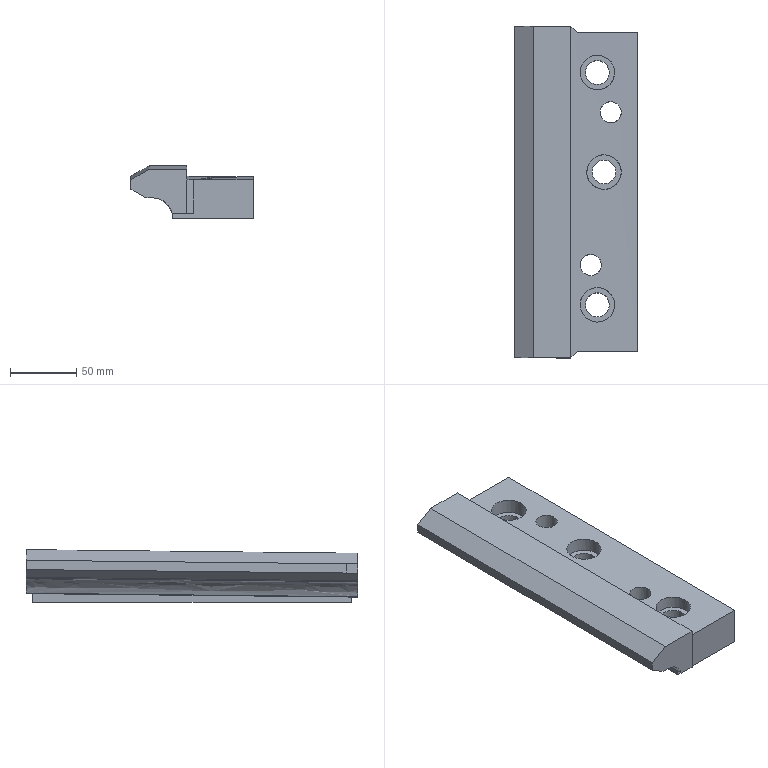Part | NX | features solid 2 | 1 solid | 33 faces | box 92.195 x 250 x 39.654 mm | volume 579481 mm3 | plane 14 | spline 11 | cylinder 8 | commonest cylinder face diameters 18 x3 26 x3 16 x2
STEP:
#1=CARTESIAN_POINT('',(719.105,10.,-45.));
#2=VERTEX_POINT('',#1);
#3=CARTESIAN_POINT('',(719.105,10.,-38.475));
#4=VERTEX_POINT('',#3);
#5=CARTESIAN_POINT('',(719.105,10.,-49.344));
#6=DIRECTION('',(0.,0.,-1.));
#7=VECTOR('',#6,1000.);
#8=LINE('',#5,#7);
#9=EDGE_CURVE('',#2,#4,#8,.F.);
#10=ORIENTED_EDGE('',*,*,#9,.F.);
#11=CARTESIAN_POINT('',(719.103,-230.,-45.));
#12=VERTEX_POINT('',#11);
#13=CARTESIAN_POINT('',(719.105,10.,-45.));
#14=CARTESIAN_POINT('',(719.108,-70.,-45.));
#15=CARTESIAN_POINT('',(719.097,-150.,-45.));
#16=CARTESIAN_POINT('',(719.103,-230.,-45.));
#17=B_SPLINE_CURVE_WITH_KNOTS('',3,(#13,#14,#15,#16),.UNSPECIFIED.,.F.,.F.,(4,4),(0.,0.24),.UNSPECIFIED.);
#18=EDGE_CURVE('',#2,#12,#17,.T.);
#19=ORIENTED_EDGE('',*,*,#18,.T.);
#20=CARTESIAN_POINT('',(719.103,-230.,-41.019));
#21=VERTEX_POINT('',#20);
#22=CARTESIAN_POINT('',(719.103,-230.,-50.615));
#23=DIRECTION('',(0.,0.,-1.));
#24=VECTOR('',#23,1000.);
#25=LINE('',#22,#24);
#26=EDGE_CURVE('',#21,#12,#25,.T.);
#27=ORIENTED_EDGE('',*,*,#26,.F.);
#28=CARTESIAN_POINT('',(719.103,-230.,-41.019));
#29=CARTESIAN_POINT('',(719.097,-149.999,-40.247));
#30=CARTESIAN_POINT('',(719.108,-69.999,-39.4));
#31=CARTESIAN_POINT('',(719.105,10.,-38.475));
#32=B_SPLINE_CURVE_WITH_KNOTS('',3,(#28,#29,#30,#31),.UNSPECIFIED.,.F.,.F.,(4,4),(0.006561,0.2466),.UNSPECIFIED.);
#33=EDGE_CURVE('',#21,#4,#32,.T.);
#34=ORIENTED_EDGE('',*,*,#33,.T.);
#35=EDGE_LOOP('',(#10,#19,#27,#34));
#36=FACE_BOUND('',#35,.T.);
#37=CARTESIAN_POINT('',(719.105,10.,-38.434));
#38=CARTESIAN_POINT('',(719.105,10.,-45.039));
#39=CARTESIAN_POINT('',(719.108,-70.005,-39.358));
#40=CARTESIAN_POINT('',(719.108,-70.005,-45.963));
#41=CARTESIAN_POINT('',(719.097,-149.999,-40.21));
#42=CARTESIAN_POINT('',(719.097,-149.999,-46.815));
#43=CARTESIAN_POINT('',(719.103,-230.,-40.978));
#44=CARTESIAN_POINT('',(719.103,-230.,-47.583));
#45=B_SPLINE_SURFACE_WITH_KNOTS('',3,1,((#37,#38),(#39,#40),(#41,#42),(#43,#44)),.SURF_OF_LINEAR_EXTRUSION.,.F.,.F.,.F.,(4,4),(2,2),(0.3477,0.6676),(0.,1.),.PIECEWISE_BEZIER_KNOTS.);
#46=ADVANCED_FACE('',(#36),#45,.F.);
#47=CARTESIAN_POINT('',(780.,10.,-45.));
#48=VERTEX_POINT('',#47);
#49=CARTESIAN_POINT('',(730.,10.,-45.));
#50=DIRECTION('',(1.,0.,0.));
#51=VECTOR('',#50,1000.);
#52=LINE('',#49,#51);
#53=EDGE_CURVE('',#2,#48,#52,.T.);
#54=ORIENTED_EDGE('',*,*,#53,.F.);
#55=ORIENTED_EDGE('',*,*,#9,.T.);
#56=CARTESIAN_POINT('',(718.904,10.,-38.359));
#57=VERTEX_POINT('',#56);
#58=CARTESIAN_POINT('',(719.105,10.,-38.475));
#59=CARTESIAN_POINT('',(719.038,10.,-38.437));
#60=CARTESIAN_POINT('',(718.971,10.,-38.398));
#61=CARTESIAN_POINT('',(718.904,10.,-38.359));
#62=B_SPLINE_CURVE_WITH_KNOTS('',3,(#58,#59,#60,#61),.UNSPECIFIED.,.F.,.F.,(4,4),(0.01267,0.0129),.UNSPECIFIED.);
#63=EDGE_CURVE('',#4,#57,#62,.T.);
#64=ORIENTED_EDGE('',*,*,#63,.T.);
#65=CARTESIAN_POINT('',(735.,10.,-38.359));
#66=VERTEX_POINT('',#65);
#67=CARTESIAN_POINT('',(669.104,10.,-38.359));
#68=DIRECTION('',(1.,0.,0.));
#69=VECTOR('',#68,1000.);
#70=LINE('',#67,#69);
#71=EDGE_CURVE('',#57,#66,#70,.T.);
#72=ORIENTED_EDGE('',*,*,#71,.T.);
#73=CARTESIAN_POINT('',(735.,10.,-13.527));
#74=VERTEX_POINT('',#73);
#75=CARTESIAN_POINT('',(735.,10.,-43.689));
#76=DIRECTION('',(0.,0.,-1.));
#77=VECTOR('',#76,1000.);
#78=LINE('',#75,#77);
#79=EDGE_CURVE('',#74,#66,#78,.T.);
#80=ORIENTED_EDGE('',*,*,#79,.F.);
#81=CARTESIAN_POINT('',(780.,10.,-13.527));
#82=VERTEX_POINT('',#81);
#83=CARTESIAN_POINT('',(754.976,10.,-13.527));
#84=DIRECTION('',(1.,0.,0.));
#85=VECTOR('',#84,1000.);
#86=LINE('',#83,#85);
#87=EDGE_CURVE('',#74,#82,#86,.T.);
#88=ORIENTED_EDGE('',*,*,#87,.T.);
#89=CARTESIAN_POINT('',(780.,10.,-5.));
#90=DIRECTION('',(0.,0.,1.));
#91=VECTOR('',#90,1000.);
#92=LINE('',#89,#91);
#93=EDGE_CURVE('',#48,#82,#92,.T.);
#94=ORIENTED_EDGE('',*,*,#93,.F.);
#95=EDGE_LOOP('',(#54,#55,#64,#72,#80,#88,#94));
#96=FACE_BOUND('',#95,.T.);
#97=CARTESIAN_POINT('',(730.,10.,-149.315));
#98=DIRECTION('',(0.,-1.,0.));
#99=DIRECTION('',(0.,0.,-1.));
#100=AXIS2_PLACEMENT_3D('',#97,#98,#99);
#101=PLANE('',#100);
#102=ADVANCED_FACE('',(#96),#101,.F.);
#103=CARTESIAN_POINT('',(780.,-230.,-45.));
#104=VERTEX_POINT('',#103);
#105=CARTESIAN_POINT('',(730.,-230.,-45.));
#106=DIRECTION('',(-1.,0.,0.));
#107=VECTOR('',#106,1000.);
#108=LINE('',#105,#107);
#109=EDGE_CURVE('',#104,#12,#108,.T.);
#110=ORIENTED_EDGE('',*,*,#109,.F.);
#111=CARTESIAN_POINT('',(780.,-230.,-16.093));
#112=VERTEX_POINT('',#111);
#113=CARTESIAN_POINT('',(780.,-230.,-5.));
#114=DIRECTION('',(0.,0.,-1.));
#115=VECTOR('',#114,1000.);
#116=LINE('',#113,#115);
#117=EDGE_CURVE('',#112,#104,#116,.T.);
#118=ORIENTED_EDGE('',*,*,#117,.F.);
#119=CARTESIAN_POINT('',(735.,-230.,-16.093));
#120=VERTEX_POINT('',#119);
#121=CARTESIAN_POINT('',(755.021,-230.,-16.093));
#122=DIRECTION('',(1.,0.,0.));
#123=VECTOR('',#122,1000.);
#124=LINE('',#121,#123);
#125=EDGE_CURVE('',#112,#120,#124,.F.);
#126=ORIENTED_EDGE('',*,*,#125,.T.);
#127=CARTESIAN_POINT('',(735.,-230.,-41.019));
#128=VERTEX_POINT('',#127);
#129=CARTESIAN_POINT('',(735.,-230.,-16.093));
#130=DIRECTION('',(0.,0.,1.));
#131=VECTOR('',#130,1000.);
#132=LINE('',#129,#131);
#133=EDGE_CURVE('',#128,#120,#132,.T.);
#134=ORIENTED_EDGE('',*,*,#133,.F.);
#135=CARTESIAN_POINT('',(669.103,-230.,-41.019));
#136=DIRECTION('',(1.,0.,0.));
#137=VECTOR('',#136,1000.);
#138=LINE('',#135,#137);
#139=EDGE_CURVE('',#21,#128,#138,.T.);
#140=ORIENTED_EDGE('',*,*,#139,.F.);
#141=ORIENTED_EDGE('',*,*,#26,.T.);
#142=EDGE_LOOP('',(#110,#118,#126,#134,#140,#141));
#143=FACE_BOUND('',#142,.T.);
#144=CARTESIAN_POINT('',(730.,-230.,49.361));
#145=DIRECTION('',(0.,1.,0.));
#146=DIRECTION('',(0.,0.,1.));
#147=AXIS2_PLACEMENT_3D('',#144,#145,#146);
#148=PLANE('',#147);
#149=ADVANCED_FACE('',(#143),#148,.F.);
#150=ORIENTED_EDGE('',*,*,#117,.T.);
#151=CARTESIAN_POINT('',(780.,-135.,-45.));
#152=DIRECTION('',(0.,1.,0.));
#153=VECTOR('',#152,1000.);
#154=LINE('',#151,#153);
#155=EDGE_CURVE('',#104,#48,#154,.T.);
#156=ORIENTED_EDGE('',*,*,#155,.T.);
#157=ORIENTED_EDGE('',*,*,#93,.T.);
#158=CARTESIAN_POINT('',(780.,10.,-13.527));
#159=CARTESIAN_POINT('',(780.,-69.999,-14.462));
#160=CARTESIAN_POINT('',(780.,-149.999,-15.327));
#161=CARTESIAN_POINT('',(780.,-230.,-16.093));
#162=B_SPLINE_CURVE_WITH_KNOTS('',3,(#158,#159,#160,#161),.UNSPECIFIED.,.F.,.F.,(4,4),(0.8306,1.071),.UNSPECIFIED.);
#163=EDGE_CURVE('',#82,#112,#162,.T.);
#164=ORIENTED_EDGE('',*,*,#163,.T.);
#165=EDGE_LOOP('',(#150,#156,#157,#164));
#166=FACE_BOUND('',#165,.T.);
#167=CARTESIAN_POINT('',(780.,-135.,-5.));
#168=DIRECTION('',(1.,0.,0.));
#169=DIRECTION('',(0.,1.,0.));
#170=AXIS2_PLACEMENT_3D('',#167,#168,#169);
#171=PLANE('',#170);
#172=ADVANCED_FACE('',(#166),#171,.T.);
#173=CARTESIAN_POINT('',(741.,-20.,-25.));
#174=VERTEX_POINT('',#173);
#175=CARTESIAN_POINT('',(750.,-20.,-25.));
#176=DIRECTION('',(0.,0.,-1.));
#177=DIRECTION('',(-1.,0.,0.));
#178=AXIS2_PLACEMENT_3D('',#175,#176,#177);
#179=CIRCLE('',#178,9.);
#180=EDGE_CURVE('',#174,#174,#179,.T.);
#181=ORIENTED_EDGE('',*,*,#180,.F.);
#182=EDGE_LOOP('',(#181));
#183=FACE_BOUND('',#182,.T.);
#184=CARTESIAN_POINT('',(741.,-20.,-45.));
#185=VERTEX_POINT('',#184);
#186=CARTESIAN_POINT('',(750.,-20.,-45.));
#187=DIRECTION('',(0.,0.,-1.));
#188=DIRECTION('',(-1.,0.,0.));
#189=AXIS2_PLACEMENT_3D('',#186,#187,#188);
#190=CIRCLE('',#189,9.);
#191=EDGE_CURVE('',#185,#185,#190,.F.);
#192=ORIENTED_EDGE('',*,*,#191,.F.);
#193=EDGE_LOOP('',(#192));
#194=FACE_BOUND('',#193,.T.);
#195=CARTESIAN_POINT('',(750.,-20.,-40.));
#196=DIRECTION('',(0.,0.,-1.));
#197=DIRECTION('',(-1.,0.,0.));
#198=AXIS2_PLACEMENT_3D('',#195,#196,#197);
#199=CYLINDRICAL_SURFACE('',#198,9.);
#200=ADVANCED_FACE('',(#183,#194),#199,.F.);
#201=CARTESIAN_POINT('',(752.044,-50.84,-14.225));
#202=VERTEX_POINT('',#201);
#203=CARTESIAN_POINT('',(754.43,-56.899,-14.293));
#204=CARTESIAN_POINT('',(751.181,-50.93,-14.226));
#205=CARTESIAN_POINT('',(753.11,-44.423,-14.153));
#206=CARTESIAN_POINT('',(759.063,-41.185,-14.116));
#207=CARTESIAN_POINT('',(765.573,-43.103,-14.138));
#208=CARTESIAN_POINT('',(768.815,-49.068,-14.205));
#209=CARTESIAN_POINT('',(766.898,-55.567,-14.278));
#210=CARTESIAN_POINT('',(760.941,-58.816,-14.314));
#211=CARTESIAN_POINT('',(754.43,-56.899,-14.293));
#212=CARTESIAN_POINT('',(751.181,-50.93,-14.226));
#213=CARTESIAN_POINT('',(753.11,-44.423,-14.153));
#214=B_SPLINE_CURVE_WITH_KNOTS('',3,(#203,#204,#205,#206,#207,#208,#209,#210,#211,#212,#213),.UNSPECIFIED.,.T.,.F.,(1,1,1,1,1,1,1,1,1,1,1,1,1,1,1),(-0.01876,-0.0125,-0.006252,0.,0.006252,0.0125,0.01876,0.02501,0.03126,0.03751,0.04377,0.05002,0.05627,0.06252,0.06878),.UNSPECIFIED.);
#215=EDGE_CURVE('',#202,#202,#214,.T.);
#216=ORIENTED_EDGE('',*,*,#215,.F.);
#217=EDGE_LOOP('',(#216));
#218=FACE_BOUND('',#217,.T.);
#219=CARTESIAN_POINT('',(752.,-50.,-45.));
#220=VERTEX_POINT('',#219);
#221=CARTESIAN_POINT('',(760.,-50.,-45.));
#222=DIRECTION('',(0.,0.,-1.));
#223=DIRECTION('',(-1.,0.,0.));
#224=AXIS2_PLACEMENT_3D('',#221,#222,#223);
#225=CIRCLE('',#224,8.);
#226=EDGE_CURVE('',#220,#220,#225,.F.);
#227=ORIENTED_EDGE('',*,*,#226,.F.);
#228=EDGE_LOOP('',(#227));
#229=FACE_BOUND('',#228,.T.);
#230=CARTESIAN_POINT('',(760.,-50.,-95.));
#231=DIRECTION('',(0.,0.,1.));
#232=DIRECTION('',(1.,0.,0.));
#233=AXIS2_PLACEMENT_3D('',#230,#231,#232);
#234=CYLINDRICAL_SURFACE('',#233,8.);
#235=ADVANCED_FACE('',(#218,#229),#234,.F.);
#236=CARTESIAN_POINT('',(746.,-95.,-25.));
#237=VERTEX_POINT('',#236);
#238=CARTESIAN_POINT('',(755.,-95.,-25.));
#239=DIRECTION('',(0.,0.,-1.));
#240=DIRECTION('',(-1.,0.,0.));
#241=AXIS2_PLACEMENT_3D('',#238,#239,#240);
#242=CIRCLE('',#241,9.);
#243=EDGE_CURVE('',#237,#237,#242,.T.);
#244=ORIENTED_EDGE('',*,*,#243,.F.);
#245=EDGE_LOOP('',(#244));
#246=FACE_BOUND('',#245,.T.);
#247=CARTESIAN_POINT('',(746.,-95.,-45.));
#248=VERTEX_POINT('',#247);
#249=CARTESIAN_POINT('',(755.,-95.,-45.));
#250=DIRECTION('',(0.,0.,-1.));
#251=DIRECTION('',(-1.,0.,0.));
#252=AXIS2_PLACEMENT_3D('',#249,#250,#251);
#253=CIRCLE('',#252,9.);
#254=EDGE_CURVE('',#248,#248,#253,.F.);
#255=ORIENTED_EDGE('',*,*,#254,.F.);
#256=EDGE_LOOP('',(#255));
#257=FACE_BOUND('',#256,.T.);
#258=CARTESIAN_POINT('',(755.,-95.,-40.));
#259=DIRECTION('',(0.,0.,-1.));
#260=DIRECTION('',(-1.,0.,0.));
#261=AXIS2_PLACEMENT_3D('',#258,#259,#260);
#262=CYLINDRICAL_SURFACE('',#261,9.);
#263=ADVANCED_FACE('',(#246,#257),#262,.F.);
#264=CARTESIAN_POINT('',(741.,-195.,-25.));
#265=VERTEX_POINT('',#264);
#266=CARTESIAN_POINT('',(750.,-195.,-25.));
#267=DIRECTION('',(0.,0.,-1.));
#268=DIRECTION('',(-1.,0.,0.));
#269=AXIS2_PLACEMENT_3D('',#266,#267,#268);
#270=CIRCLE('',#269,9.);
#271=EDGE_CURVE('',#265,#265,#270,.T.);
#272=ORIENTED_EDGE('',*,*,#271,.F.);
#273=EDGE_LOOP('',(#272));
#274=FACE_BOUND('',#273,.T.);
#275=CARTESIAN_POINT('',(741.,-195.,-45.));
#276=VERTEX_POINT('',#275);
#277=CARTESIAN_POINT('',(750.,-195.,-45.));
#278=DIRECTION('',(0.,0.,-1.));
#279=DIRECTION('',(-1.,0.,0.));
#280=AXIS2_PLACEMENT_3D('',#277,#278,#279);
#281=CIRCLE('',#280,9.);
#282=EDGE_CURVE('',#276,#276,#281,.F.);
#283=ORIENTED_EDGE('',*,*,#282,.F.);
#284=EDGE_LOOP('',(#283));
#285=FACE_BOUND('',#284,.T.);
#286=CARTESIAN_POINT('',(750.,-195.,-40.));
#287=DIRECTION('',(0.,0.,-1.));
#288=DIRECTION('',(-1.,0.,0.));
#289=AXIS2_PLACEMENT_3D('',#286,#287,#288);
#290=CYLINDRICAL_SURFACE('',#289,9.);
#291=ADVANCED_FACE('',(#274,#285),#290,.F.);
#292=CARTESIAN_POINT('',(737.044,-165.842,-15.459));
#293=VERTEX_POINT('',#292);
#294=CARTESIAN_POINT('',(739.431,-171.9,-15.52));
#295=CARTESIAN_POINT('',(736.182,-165.931,-15.46));
#296=CARTESIAN_POINT('',(738.109,-159.425,-15.393));
#297=CARTESIAN_POINT('',(744.061,-156.186,-15.36));
#298=CARTESIAN_POINT('',(750.572,-158.102,-15.379));
#299=CARTESIAN_POINT('',(753.815,-164.066,-15.441));
#300=CARTESIAN_POINT('',(751.899,-170.566,-15.507));
#301=CARTESIAN_POINT('',(745.942,-173.816,-15.54));
#302=CARTESIAN_POINT('',(739.431,-171.9,-15.52));
#303=CARTESIAN_POINT('',(736.182,-165.931,-15.46));
#304=CARTESIAN_POINT('',(738.109,-159.425,-15.393));
#305=B_SPLINE_CURVE_WITH_KNOTS('',3,(#294,#295,#296,#297,#298,#299,#300,#301,#302,#303,#304),.UNSPECIFIED.,.T.,.F.,(1,1,1,1,1,1,1,1,1,1,1,1,1,1,1),(-0.01876,-0.0125,-0.006252,0.,0.006252,0.0125,0.01876,0.02501,0.03126,0.03751,0.04377,0.05002,0.05627,0.06252,0.06878),.UNSPECIFIED.);
#306=EDGE_CURVE('',#293,#293,#305,.T.);
#307=ORIENTED_EDGE('',*,*,#306,.F.);
#308=EDGE_LOOP('',(#307));
#309=FACE_BOUND('',#308,.T.);
#310=CARTESIAN_POINT('',(737.,-165.,-45.));
#311=VERTEX_POINT('',#310);
#312=CARTESIAN_POINT('',(745.,-165.,-45.));
#313=DIRECTION('',(0.,0.,-1.));
#314=DIRECTION('',(-1.,0.,0.));
#315=AXIS2_PLACEMENT_3D('',#312,#313,#314);
#316=CIRCLE('',#315,8.);
#317=EDGE_CURVE('',#311,#311,#316,.F.);
#318=ORIENTED_EDGE('',*,*,#317,.F.);
#319=EDGE_LOOP('',(#318));
#320=FACE_BOUND('',#319,.T.);
#321=CARTESIAN_POINT('',(745.,-165.,-95.));
#322=DIRECTION('',(0.,0.,1.));
#323=DIRECTION('',(1.,0.,0.));
#324=AXIS2_PLACEMENT_3D('',#321,#322,#323);
#325=CYLINDRICAL_SURFACE('',#324,8.);
#326=ADVANCED_FACE('',(#309,#320),#325,.F.);
#327=CARTESIAN_POINT('',(730.,-235.,-41.019));
#328=VERTEX_POINT('',#327);
#329=CARTESIAN_POINT('',(730.,-235.,-16.141));
#330=VERTEX_POINT('',#329);
#331=CARTESIAN_POINT('',(730.,-235.,-50.));
#332=DIRECTION('',(0.,0.,-1.));
#333=VECTOR('',#332,1000.);
#334=LINE('',#331,#333);
#335=EDGE_CURVE('',#328,#330,#334,.F.);
#336=ORIENTED_EDGE('',*,*,#335,.F.);
#337=CARTESIAN_POINT('',(730.,-235.,-41.019));
#338=DIRECTION('',(0.7071,0.7071,0.));
#339=VECTOR('',#338,1000.);
#340=LINE('',#337,#339);
#341=EDGE_CURVE('',#328,#128,#340,.T.);
#342=ORIENTED_EDGE('',*,*,#341,.T.);
#343=ORIENTED_EDGE('',*,*,#133,.T.);
#344=CARTESIAN_POINT('',(735.,-230.,-16.093));
#345=CARTESIAN_POINT('',(733.333,-231.667,-16.109));
#346=CARTESIAN_POINT('',(731.667,-233.333,-16.125));
#347=CARTESIAN_POINT('',(730.,-235.,-16.141));
#348=B_SPLINE_CURVE_WITH_KNOTS('',3,(#344,#345,#346,#347),.UNSPECIFIED.,.F.,.F.,(4,4),(0.,0.007071),.UNSPECIFIED.);
#349=EDGE_CURVE('',#120,#330,#348,.T.);
#350=ORIENTED_EDGE('',*,*,#349,.T.);
#351=EDGE_LOOP('',(#336,#342,#343,#350));
#352=FACE_BOUND('',#351,.T.);
#353=CARTESIAN_POINT('',(730.,-235.,-50.));
#354=DIRECTION('',(0.7071,-0.7071,0.));
#355=DIRECTION('',(-0.7071,-0.7071,0.));
#356=AXIS2_PLACEMENT_3D('',#353,#354,#355);
#357=PLANE('',#356);
#358=ADVANCED_FACE('',(#352),#357,.T.);
#359=ORIENTED_EDGE('',*,*,#341,.F.);
#360=CARTESIAN_POINT('',(719.02,-235.,-41.019));
#361=VERTEX_POINT('',#360);
#362=CARTESIAN_POINT('',(675.,-235.,-41.019));
#363=DIRECTION('',(-1.,0.,0.));
#364=VECTOR('',#363,1000.);
#365=LINE('',#362,#364);
#366=EDGE_CURVE('',#361,#328,#365,.F.);
#367=ORIENTED_EDGE('',*,*,#366,.F.);
#368=CARTESIAN_POINT('',(719.103,-230.,-41.019));
#369=CARTESIAN_POINT('',(719.075,-231.667,-41.019));
#370=CARTESIAN_POINT('',(719.047,-233.333,-41.019));
#371=CARTESIAN_POINT('',(719.02,-235.,-41.019));
#372=B_SPLINE_CURVE_WITH_KNOTS('',3,(#368,#369,#370,#371),.UNSPECIFIED.,.F.,.F.,(4,4),(0.,0.005001),.UNSPECIFIED.);
#373=EDGE_CURVE('',#21,#361,#372,.T.);
#374=ORIENTED_EDGE('',*,*,#373,.F.);
#375=ORIENTED_EDGE('',*,*,#139,.T.);
#376=EDGE_LOOP('',(#359,#367,#374,#375));
#377=FACE_BOUND('',#376,.T.);
#378=CARTESIAN_POINT('',(669.103,-230.,-41.019));
#379=DIRECTION('',(0.,0.,-1.));
#380=DIRECTION('',(1.,0.,0.));
#381=AXIS2_PLACEMENT_3D('',#378,#379,#380);
#382=PLANE('',#381);
#383=ADVANCED_FACE('',(#377),#382,.T.);
#384=CARTESIAN_POINT('',(730.,15.,-38.359));
#385=VERTEX_POINT('',#384);
#386=CARTESIAN_POINT('',(730.,15.,-38.359));
#387=DIRECTION('',(0.7071,-0.7071,0.));
#388=VECTOR('',#387,1000.);
#389=LINE('',#386,#388);
#390=EDGE_CURVE('',#385,#66,#389,.T.);
#391=ORIENTED_EDGE('',*,*,#390,.F.);
#392=CARTESIAN_POINT('',(730.,15.,-13.468));
#393=VERTEX_POINT('',#392);
#394=CARTESIAN_POINT('',(730.,15.,-50.));
#395=DIRECTION('',(0.,0.,-1.));
#396=VECTOR('',#395,1000.);
#397=LINE('',#394,#396);
#398=EDGE_CURVE('',#393,#385,#397,.T.);
#399=ORIENTED_EDGE('',*,*,#398,.F.);
#400=CARTESIAN_POINT('',(730.,15.,-13.468));
#401=CARTESIAN_POINT('',(731.667,13.333,-13.488));
#402=CARTESIAN_POINT('',(733.333,11.667,-13.507));
#403=CARTESIAN_POINT('',(735.,10.,-13.527));
#404=B_SPLINE_CURVE_WITH_KNOTS('',3,(#400,#401,#402,#403),.UNSPECIFIED.,.F.,.F.,(4,4),(0.,0.007071),.UNSPECIFIED.);
#405=EDGE_CURVE('',#393,#74,#404,.T.);
#406=ORIENTED_EDGE('',*,*,#405,.T.);
#407=ORIENTED_EDGE('',*,*,#79,.T.);
#408=EDGE_LOOP('',(#391,#399,#406,#407));
#409=FACE_BOUND('',#408,.T.);
#410=CARTESIAN_POINT('',(730.,15.,-50.));
#411=DIRECTION('',(0.7071,0.7071,0.));
#412=DIRECTION('',(0.7071,-0.7071,0.));
#413=AXIS2_PLACEMENT_3D('',#410,#411,#412);
#414=PLANE('',#413);
#415=ADVANCED_FACE('',(#409),#414,.T.);
#416=ORIENTED_EDGE('',*,*,#33,.F.);
#417=ORIENTED_EDGE('',*,*,#373,.T.);
#418=CARTESIAN_POINT('',(718.634,-235.,-40.796));
#419=VERTEX_POINT('',#418);
#420=CARTESIAN_POINT('',(718.634,-235.,-40.796));
#421=CARTESIAN_POINT('',(718.763,-235.,-40.87));
#422=CARTESIAN_POINT('',(718.891,-235.,-40.945));
#423=CARTESIAN_POINT('',(719.02,-235.,-41.019));
#424=B_SPLINE_CURVE_WITH_KNOTS('',3,(#420,#421,#422,#423),.UNSPECIFIED.,.F.,.F.,(4,4),(0.02431,0.02476),.UNSPECIFIED.);
#425=EDGE_CURVE('',#419,#361,#424,.T.);
#426=ORIENTED_EDGE('',*,*,#425,.F.);
#427=CARTESIAN_POINT('',(718.635,15.,-38.146));
#428=VERTEX_POINT('',#427);
#429=CARTESIAN_POINT('',(718.634,-235.,-40.796));
#430=CARTESIAN_POINT('',(718.627,-151.666,-39.995));
#431=CARTESIAN_POINT('',(718.64,-68.332,-39.113));
#432=CARTESIAN_POINT('',(718.635,15.,-38.146));
#433=B_SPLINE_CURVE_WITH_KNOTS('',3,(#429,#430,#431,#432),.UNSPECIFIED.,.F.,.F.,(4,4),(0.001564,0.2516),.UNSPECIFIED.);
#434=EDGE_CURVE('',#419,#428,#433,.T.);
#435=ORIENTED_EDGE('',*,*,#434,.T.);
#436=CARTESIAN_POINT('',(719.004,15.,-38.359));
#437=VERTEX_POINT('',#436);
#438=CARTESIAN_POINT('',(719.004,15.,-38.359));
#439=CARTESIAN_POINT('',(718.881,15.,-38.288));
#440=CARTESIAN_POINT('',(718.758,15.,-38.217));
#441=CARTESIAN_POINT('',(718.635,15.,-38.146));
#442=B_SPLINE_CURVE_WITH_KNOTS('',3,(#438,#439,#440,#441),.UNSPECIFIED.,.F.,.F.,(4,4),(0.0127,0.01312),.UNSPECIFIED.);
#443=EDGE_CURVE('',#437,#428,#442,.T.);
#444=ORIENTED_EDGE('',*,*,#443,.F.);
#445=CARTESIAN_POINT('',(718.904,10.,-38.359));
#446=CARTESIAN_POINT('',(718.937,11.667,-38.359));
#447=CARTESIAN_POINT('',(718.971,13.333,-38.359));
#448=CARTESIAN_POINT('',(719.004,15.,-38.359));
#449=B_SPLINE_CURVE_WITH_KNOTS('',3,(#445,#446,#447,#448),.UNSPECIFIED.,.F.,.F.,(4,4),(0.,0.005001),.UNSPECIFIED.);
#450=EDGE_CURVE('',#57,#437,#449,.T.);
#451=ORIENTED_EDGE('',*,*,#450,.F.);
#452=ORIENTED_EDGE('',*,*,#63,.F.);
#453=EDGE_LOOP('',(#416,#417,#426,#435,#444,#451,#452));
#454=FACE_BOUND('',#453,.T.);
#455=CARTESIAN_POINT('',(718.632,16.5,-38.127));
#456=CARTESIAN_POINT('',(719.112,16.503,-38.404));
#457=CARTESIAN_POINT('',(718.632,-1.249,-38.333));
#458=CARTESIAN_POINT('',(719.112,-1.246,-38.61));
#459=CARTESIAN_POINT('',(718.629,-47.43,-38.858));
#460=CARTESIAN_POINT('',(719.109,-47.427,-39.135));
#461=CARTESIAN_POINT('',(718.622,-131.769,-39.773));
#462=CARTESIAN_POINT('',(719.102,-131.766,-40.05));
#463=CARTESIAN_POINT('',(718.624,-198.349,-40.441));
#464=CARTESIAN_POINT('',(719.104,-198.346,-40.718));
#465=CARTESIAN_POINT('',(718.626,-236.502,-40.806));
#466=CARTESIAN_POINT('',(719.106,-236.499,-41.083));
#467=B_SPLINE_SURFACE_WITH_KNOTS('',3,1,((#455,#456),(#457,#458),(#459,#460),(#461,#462),(#463,#464),(#465,#466)),.RULED_SURF.,.F.,.F.,.F.,(4,1,1,4),(2,2),(0.2969,0.375,0.5,0.6678),(0.9567,0.9785),.UNSPECIFIED.);
#468=ADVANCED_FACE('',(#454),#467,.F.);
#469=CARTESIAN_POINT('',(699.103,15.,-26.87));
#470=VERTEX_POINT('',#469);
#471=CARTESIAN_POINT('',(699.103,-235.,-29.518));
#472=VERTEX_POINT('',#471);
#473=CARTESIAN_POINT('',(699.103,-235.,-29.519));
#474=CARTESIAN_POINT('',(699.098,-151.666,-28.72));
#475=CARTESIAN_POINT('',(699.106,-68.332,-27.836));
#476=CARTESIAN_POINT('',(699.105,15.,-26.87));
#477=B_SPLINE_CURVE_WITH_KNOTS('',3,(#473,#474,#475,#476),.UNSPECIFIED.,.F.,.F.,(4,4),(0.,1.),.UNSPECIFIED.);
#478=EDGE_CURVE('',#470,#472,#477,.F.);
#479=ORIENTED_EDGE('',*,*,#478,.T.);
#480=CARTESIAN_POINT('',(697.581,-235.,-28.641));
#481=VERTEX_POINT('',#480);
#482=CARTESIAN_POINT('',(697.581,-235.,-28.641));
#483=CARTESIAN_POINT('',(698.088,-235.,-28.933));
#484=CARTESIAN_POINT('',(698.595,-235.,-29.226));
#485=CARTESIAN_POINT('',(699.102,-235.,-29.518));
#486=B_SPLINE_CURVE_WITH_KNOTS('',3,(#482,#483,#484,#485),.UNSPECIFIED.,.F.,.F.,(4,4),(0.,0.001756),.UNSPECIFIED.);
#487=EDGE_CURVE('',#481,#472,#486,.T.);
#488=ORIENTED_EDGE('',*,*,#487,.F.);
#489=CARTESIAN_POINT('',(697.587,15.,-25.994));
#490=VERTEX_POINT('',#489);
#491=CARTESIAN_POINT('',(697.581,-235.,-28.641));
#492=CARTESIAN_POINT('',(697.578,-151.666,-27.842));
#493=CARTESIAN_POINT('',(697.587,-68.332,-26.959));
#494=CARTESIAN_POINT('',(697.587,15.,-25.994));
#495=B_SPLINE_CURVE_WITH_KNOTS('',3,(#491,#492,#493,#494),.UNSPECIFIED.,.F.,.F.,(4,4),(0.3346,0.7011),.UNSPECIFIED.);
#496=EDGE_CURVE('',#490,#481,#495,.F.);
#497=ORIENTED_EDGE('',*,*,#496,.F.);
#498=CARTESIAN_POINT('',(699.104,15.,-26.87));
#499=CARTESIAN_POINT('',(698.599,15.,-26.578));
#500=CARTESIAN_POINT('',(698.093,15.,-26.286));
#501=CARTESIAN_POINT('',(697.587,15.,-25.994));
#502=B_SPLINE_CURVE_WITH_KNOTS('',3,(#498,#499,#500,#501),.UNSPECIFIED.,.F.,.F.,(4,4),(0.03568,0.03743),.UNSPECIFIED.);
#503=EDGE_CURVE('',#470,#490,#502,.T.);
#504=ORIENTED_EDGE('',*,*,#503,.F.);
#505=EDGE_LOOP('',(#479,#488,#497,#504));
#506=FACE_BOUND('',#505,.T.);
#507=CARTESIAN_POINT('',(697.587,16.5,-25.977));
#508=CARTESIAN_POINT('',(699.119,16.511,-26.861));
#509=CARTESIAN_POINT('',(697.587,-1.298,-26.183));
#510=CARTESIAN_POINT('',(699.118,-1.287,-27.067));
#511=CARTESIAN_POINT('',(697.585,-47.52,-26.709));
#512=CARTESIAN_POINT('',(699.116,-47.51,-27.593));
#513=CARTESIAN_POINT('',(697.577,-131.856,-27.623));
#514=CARTESIAN_POINT('',(699.109,-131.847,-28.507));
#515=CARTESIAN_POINT('',(697.58,-198.395,-28.29));
#516=CARTESIAN_POINT('',(699.111,-198.386,-29.174));
#517=CARTESIAN_POINT('',(697.581,-236.508,-28.655));
#518=CARTESIAN_POINT('',(699.112,-236.5,-29.539));
#519=B_SPLINE_SURFACE_WITH_KNOTS('',3,1,((#507,#508),(#509,#510),(#511,#512),(#513,#514),(#515,#516),(#517,#518)),.RULED_SURF.,.F.,.F.,.F.,(4,1,1,4),(2,2),(0.2967,0.375,0.5,0.6676),(0.000000001,0.06961),.UNSPECIFIED.);
#520=ADVANCED_FACE('',(#506),#519,.F.);
#521=ORIENTED_EDGE('',*,*,#366,.T.);
#522=ORIENTED_EDGE('',*,*,#335,.T.);
#523=CARTESIAN_POINT('',(730.,-235.,-8.022));
#524=VERTEX_POINT('',#523);
#525=CARTESIAN_POINT('',(730.,-235.,-50.));
#526=DIRECTION('',(0.,0.,1.));
#527=VECTOR('',#526,1000.);
#528=LINE('',#525,#527);
#529=EDGE_CURVE('',#330,#524,#528,.T.);
#530=ORIENTED_EDGE('',*,*,#529,.T.);
#531=CARTESIAN_POINT('',(701.709,-235.,-8.022));
#532=VERTEX_POINT('',#531);
#533=CARTESIAN_POINT('',(708.926,-235.,-8.022));
#534=DIRECTION('',(1.,0.,0.));
#535=VECTOR('',#534,1000.);
#536=LINE('',#533,#535);
#537=EDGE_CURVE('',#532,#524,#536,.T.);
#538=ORIENTED_EDGE('',*,*,#537,.F.);
#539=CARTESIAN_POINT('',(687.852,-235.,-16.023));
#540=VERTEX_POINT('',#539);
#541=CARTESIAN_POINT('',(601.249,-235.,-66.023));
#542=DIRECTION('',(0.866,0.,0.5));
#543=VECTOR('',#542,1000.);
#544=LINE('',#541,#543);
#545=EDGE_CURVE('',#540,#532,#544,.T.);
#546=ORIENTED_EDGE('',*,*,#545,.F.);
#547=CARTESIAN_POINT('',(687.852,-235.,-23.023));
#548=VERTEX_POINT('',#547);
#549=CARTESIAN_POINT('',(687.852,-235.,-19.587));
#550=DIRECTION('',(0.,0.,-1.));
#551=VECTOR('',#550,1000.);
#552=LINE('',#549,#551);
#553=EDGE_CURVE('',#548,#540,#552,.F.);
#554=ORIENTED_EDGE('',*,*,#553,.F.);
#555=CARTESIAN_POINT('',(687.852,-235.,-23.023));
#556=CARTESIAN_POINT('',(691.095,-235.,-24.896));
#557=CARTESIAN_POINT('',(694.338,-235.,-26.768));
#558=CARTESIAN_POINT('',(697.581,-235.,-28.641));
#559=B_SPLINE_CURVE_WITH_KNOTS('',3,(#555,#556,#557,#558),.UNSPECIFIED.,.F.,.F.,(4,4),(0.,0.01123),.UNSPECIFIED.);
#560=EDGE_CURVE('',#548,#481,#559,.T.);
#561=ORIENTED_EDGE('',*,*,#560,.T.);
#562=ORIENTED_EDGE('',*,*,#487,.T.);
#563=CARTESIAN_POINT('',(704.103,-235.,-29.517));
#564=VERTEX_POINT('',#563);
#565=CARTESIAN_POINT('',(704.103,-235.,-29.517));
#566=CARTESIAN_POINT('',(702.437,-235.,-29.517));
#567=CARTESIAN_POINT('',(700.771,-235.,-29.517));
#568=CARTESIAN_POINT('',(699.105,-235.,-29.517));
#569=B_SPLINE_CURVE_WITH_KNOTS('',3,(#565,#566,#567,#568),.UNSPECIFIED.,.F.,.F.,(4,4),(0.00003872,0.005037),.UNSPECIFIED.);
#570=EDGE_CURVE('',#564,#472,#569,.T.);
#571=ORIENTED_EDGE('',*,*,#570,.F.);
#572=CARTESIAN_POINT('',(704.103,-235.,-29.517));
#573=CARTESIAN_POINT('',(707.436,-235.,-29.517));
#574=CARTESIAN_POINT('',(713.977,-235.,-31.786));
#575=CARTESIAN_POINT('',(717.811,-235.,-37.583));
#576=CARTESIAN_POINT('',(718.634,-235.,-40.796));
#577=B_SPLINE_CURVE_WITH_KNOTS('',3,(#572,#573,#574,#575,#576),.UNSPECIFIED.,.F.,.F.,(4,1,4),(0.,0.009855,0.01971),.UNSPECIFIED.);
#578=EDGE_CURVE('',#564,#419,#577,.T.);
#579=ORIENTED_EDGE('',*,*,#578,.T.);
#580=ORIENTED_EDGE('',*,*,#425,.T.);
#581=EDGE_LOOP('',(#521,#522,#530,#538,#546,#554,#561,#562,#571,#579,#580));
#582=FACE_BOUND('',#581,.T.);
#583=CARTESIAN_POINT('',(675.,-235.,200.));
#584=DIRECTION('',(0.,1.,0.));
#585=DIRECTION('',(0.,0.,1.));
#586=AXIS2_PLACEMENT_3D('',#583,#584,#585);
#587=PLANE('',#586);
#588=ADVANCED_FACE('',(#582),#587,.F.);
#589=CARTESIAN_POINT('',(719.105,15.,-37.908));
#590=VERTEX_POINT('',#589);
#591=CARTESIAN_POINT('',(719.105,15.,-13.468));
#592=VERTEX_POINT('',#591);
#593=CARTESIAN_POINT('',(719.105,15.,-34.204));
#594=DIRECTION('',(0.,0.,-1.));
#595=VECTOR('',#594,1000.);
#596=LINE('',#593,#595);
#597=EDGE_CURVE('',#590,#592,#596,.F.);
#598=ORIENTED_EDGE('',*,*,#597,.T.);
#599=ORIENTED_EDGE('',*,*,#597,.F.);
#600=EDGE_LOOP('',(#598,#599));
#601=FACE_BOUND('',#600,.T.);
#602=ORIENTED_EDGE('',*,*,#398,.T.);
#603=CARTESIAN_POINT('',(734.776,15.,-38.359));
#604=DIRECTION('',(-1.,0.,0.));
#605=VECTOR('',#604,1000.);
#606=LINE('',#603,#605);
#607=EDGE_CURVE('',#437,#385,#606,.F.);
#608=ORIENTED_EDGE('',*,*,#607,.F.);
#609=ORIENTED_EDGE('',*,*,#443,.T.);
#610=CARTESIAN_POINT('',(704.105,15.,-26.87));
#611=VERTEX_POINT('',#610);
#612=CARTESIAN_POINT('',(718.635,15.,-38.146));
#613=CARTESIAN_POINT('',(717.818,15.,-34.958));
#614=CARTESIAN_POINT('',(713.994,15.,-29.139));
#615=CARTESIAN_POINT('',(707.432,15.,-26.87));
#616=CARTESIAN_POINT('',(704.105,15.,-26.87));
#617=B_SPLINE_CURVE_WITH_KNOTS('',3,(#612,#613,#614,#615,#616),.UNSPECIFIED.,.F.,.F.,(4,1,4),(0.003751,0.01359,0.02343),.UNSPECIFIED.);
#618=EDGE_CURVE('',#428,#611,#617,.T.);
#619=ORIENTED_EDGE('',*,*,#618,.T.);
#620=CARTESIAN_POINT('',(699.099,15.,-26.87));
#621=CARTESIAN_POINT('',(700.768,15.,-26.87));
#622=CARTESIAN_POINT('',(702.436,15.,-26.87));
#623=CARTESIAN_POINT('',(704.105,15.,-26.87));
#624=B_SPLINE_CURVE_WITH_KNOTS('',3,(#620,#621,#622,#623),.UNSPECIFIED.,.F.,.F.,(4,4),(0.,0.005005),.UNSPECIFIED.);
#625=EDGE_CURVE('',#470,#611,#624,.T.);
#626=ORIENTED_EDGE('',*,*,#625,.F.);
#627=ORIENTED_EDGE('',*,*,#503,.T.);
#628=CARTESIAN_POINT('',(687.805,15.,-20.347));
#629=VERTEX_POINT('',#628);
#630=CARTESIAN_POINT('',(697.587,15.,-25.994));
#631=CARTESIAN_POINT('',(694.327,15.,-24.112));
#632=CARTESIAN_POINT('',(691.066,15.,-22.229));
#633=CARTESIAN_POINT('',(687.805,15.,-20.347));
#634=B_SPLINE_CURVE_WITH_KNOTS('',3,(#630,#631,#632,#633),.UNSPECIFIED.,.F.,.F.,(4,4),(0.,0.0113),.UNSPECIFIED.);
#635=EDGE_CURVE('',#490,#629,#634,.T.);
#636=ORIENTED_EDGE('',*,*,#635,.T.);
#637=CARTESIAN_POINT('',(687.805,15.,-13.347));
#638=VERTEX_POINT('',#637);
#639=CARTESIAN_POINT('',(687.805,15.,-17.29));
#640=DIRECTION('',(0.,0.,-1.));
#641=VECTOR('',#640,1000.);
#642=LINE('',#639,#641);
#643=EDGE_CURVE('',#638,#629,#642,.T.);
#644=ORIENTED_EDGE('',*,*,#643,.F.);
#645=CARTESIAN_POINT('',(701.663,15.,-5.346));
#646=VERTEX_POINT('',#645);
#647=CARTESIAN_POINT('',(601.203,15.,-63.346));
#648=DIRECTION('',(0.866,0.,0.5));
#649=VECTOR('',#648,1000.);
#650=LINE('',#647,#649);
#651=EDGE_CURVE('',#646,#638,#650,.F.);
#652=ORIENTED_EDGE('',*,*,#651,.F.);
#653=CARTESIAN_POINT('',(730.,15.,-5.346));
#654=VERTEX_POINT('',#653);
#655=CARTESIAN_POINT('',(708.903,15.,-5.346));
#656=DIRECTION('',(1.,0.,0.));
#657=VECTOR('',#656,1000.);
#658=LINE('',#655,#657);
#659=EDGE_CURVE('',#654,#646,#658,.F.);
#660=ORIENTED_EDGE('',*,*,#659,.F.);
#661=CARTESIAN_POINT('',(730.,15.,-50.));
#662=DIRECTION('',(0.,0.,-1.));
#663=VECTOR('',#662,1000.);
#664=LINE('',#661,#663);
#665=EDGE_CURVE('',#654,#393,#664,.T.);
#666=ORIENTED_EDGE('',*,*,#665,.T.);
#667=EDGE_LOOP('',(#602,#608,#609,#619,#626,#627,#636,#644,#652,#660,#666));
#668=FACE_BOUND('',#667,.T.);
#669=CARTESIAN_POINT('',(734.776,15.,-34.57));
#670=DIRECTION('',(0.,-1.,0.));
#671=DIRECTION('',(0.,0.,-1.));
#672=AXIS2_PLACEMENT_3D('',#669,#670,#671);
#673=PLANE('',#672);
#674=ADVANCED_FACE('',(#601,#668),#673,.F.);
#675=CARTESIAN_POINT('',(737.072,-21.365,-13.89));
#676=VERTEX_POINT('',#675);
#677=CARTESIAN_POINT('',(740.948,-31.211,-14.003));
#678=CARTESIAN_POINT('',(735.67,-21.511,-13.892));
#679=CARTESIAN_POINT('',(738.804,-10.938,-13.77));
#680=CARTESIAN_POINT('',(748.476,-5.676,-13.709));
#681=CARTESIAN_POINT('',(759.056,-8.793,-13.745));
#682=CARTESIAN_POINT('',(764.325,-18.485,-13.857));
#683=CARTESIAN_POINT('',(761.209,-29.046,-13.978));
#684=CARTESIAN_POINT('',(751.529,-34.326,-14.038));
#685=CARTESIAN_POINT('',(740.948,-31.211,-14.003));
#686=CARTESIAN_POINT('',(735.67,-21.511,-13.892));
#687=CARTESIAN_POINT('',(738.804,-10.938,-13.77));
#688=B_SPLINE_CURVE_WITH_KNOTS('',3,(#677,#678,#679,#680,#681,#682,#683,#684,#685,#686,#687),.UNSPECIFIED.,.T.,.F.,(1,1,1,1,1,1,1,1,1,1,1,1,1,1,1),(-0.03048,-0.02032,-0.01016,0.,0.01016,0.02032,0.03048,0.04064,0.0508,0.06096,0.07112,0.08128,0.09144,0.1016,0.1118),.UNSPECIFIED.);
#689=EDGE_CURVE('',#676,#676,#688,.T.);
#690=ORIENTED_EDGE('',*,*,#689,.T.);
#691=EDGE_LOOP('',(#690));
#692=FACE_BOUND('',#691,.T.);
#693=ORIENTED_EDGE('',*,*,#215,.T.);
#694=EDGE_LOOP('',(#693));
#695=FACE_BOUND('',#694,.T.);
#696=CARTESIAN_POINT('',(767.713,-92.285,-14.683));
#697=VERTEX_POINT('',#696);
#698=CARTESIAN_POINT('',(762.825,-82.901,-14.581));
#699=CARTESIAN_POINT('',(769.092,-91.994,-14.68));
#700=CARTESIAN_POINT('',(767.085,-102.837,-14.798));
#701=CARTESIAN_POINT('',(758.019,-109.085,-14.865));
#702=CARTESIAN_POINT('',(747.17,-107.096,-14.844));
#703=CARTESIAN_POINT('',(740.913,-98.01,-14.746));
#704=CARTESIAN_POINT('',(742.903,-87.18,-14.628));
#705=CARTESIAN_POINT('',(751.976,-80.914,-14.559));
#706=CARTESIAN_POINT('',(762.825,-82.901,-14.581));
#707=CARTESIAN_POINT('',(769.092,-91.994,-14.68));
#708=CARTESIAN_POINT('',(767.085,-102.837,-14.798));
#709=B_SPLINE_CURVE_WITH_KNOTS('',3,(#698,#699,#700,#701,#702,#703,#704,#705,#706,#707,#708),.UNSPECIFIED.,.T.,.F.,(1,1,1,1,1,1,1,1,1,1,1,1,1,1,1),(-0.03048,-0.02032,-0.01016,0.,0.01016,0.02032,0.03048,0.04064,0.0508,0.06096,0.07112,0.08128,0.09144,0.1016,0.1118),.UNSPECIFIED.);
#710=EDGE_CURVE('',#697,#697,#709,.T.);
#711=ORIENTED_EDGE('',*,*,#710,.T.);
#712=EDGE_LOOP('',(#711));
#713=FACE_BOUND('',#712,.T.);
#714=CARTESIAN_POINT('',(737.072,-196.367,-15.765));
#715=VERTEX_POINT('',#714);
#716=CARTESIAN_POINT('',(740.95,-206.212,-15.862));
#717=CARTESIAN_POINT('',(735.67,-196.513,-15.767));
#718=CARTESIAN_POINT('',(738.803,-185.939,-15.662));
#719=CARTESIAN_POINT('',(748.475,-180.676,-15.609));
#720=CARTESIAN_POINT('',(759.055,-183.792,-15.64));
#721=CARTESIAN_POINT('',(764.325,-193.483,-15.737));
#722=CARTESIAN_POINT('',(761.21,-204.045,-15.841));
#723=CARTESIAN_POINT('',(751.531,-209.325,-15.893));
#724=CARTESIAN_POINT('',(740.95,-206.212,-15.862));
#725=CARTESIAN_POINT('',(735.67,-196.513,-15.767));
#726=CARTESIAN_POINT('',(738.803,-185.939,-15.662));
#727=B_SPLINE_CURVE_WITH_KNOTS('',3,(#716,#717,#718,#719,#720,#721,#722,#723,#724,#725,#726),.UNSPECIFIED.,.T.,.F.,(1,1,1,1,1,1,1,1,1,1,1,1,1,1,1),(-0.03048,-0.02032,-0.01016,0.,0.01016,0.02032,0.03048,0.04064,0.0508,0.06096,0.07112,0.08128,0.09144,0.1016,0.1118),.UNSPECIFIED.);
#728=EDGE_CURVE('',#715,#715,#727,.T.);
#729=ORIENTED_EDGE('',*,*,#728,.T.);
#730=EDGE_LOOP('',(#729));
#731=FACE_BOUND('',#730,.T.);
#732=ORIENTED_EDGE('',*,*,#306,.T.);
#733=EDGE_LOOP('',(#732));
#734=FACE_BOUND('',#733,.T.);
#735=CARTESIAN_POINT('',(730.,-235.,-16.141));
#736=CARTESIAN_POINT('',(730.,-151.666,-15.347));
#737=CARTESIAN_POINT('',(730.,-68.332,-14.445));
#738=CARTESIAN_POINT('',(730.,15.,-13.468));
#739=B_SPLINE_CURVE_WITH_KNOTS('',3,(#735,#736,#737,#738),.UNSPECIFIED.,.F.,.F.,(4,4),(0.,0.25),.UNSPECIFIED.);
#740=EDGE_CURVE('',#330,#393,#739,.T.);
#741=ORIENTED_EDGE('',*,*,#740,.F.);
#742=ORIENTED_EDGE('',*,*,#349,.F.);
#743=ORIENTED_EDGE('',*,*,#125,.F.);
#744=ORIENTED_EDGE('',*,*,#163,.F.);
#745=ORIENTED_EDGE('',*,*,#87,.F.);
#746=ORIENTED_EDGE('',*,*,#405,.F.);
#747=EDGE_LOOP('',(#741,#742,#743,#744,#745,#746));
#748=FACE_BOUND('',#747,.T.);
#749=CARTESIAN_POINT('',(729.648,16.5,-13.451));
#750=CARTESIAN_POINT('',(780.299,16.5,-13.451));
#751=CARTESIAN_POINT('',(729.665,-67.832,-14.44));
#752=CARTESIAN_POINT('',(780.316,-67.832,-14.44));
#753=CARTESIAN_POINT('',(729.705,-152.165,-15.353));
#754=CARTESIAN_POINT('',(780.355,-152.165,-15.353));
#755=CARTESIAN_POINT('',(729.695,-236.5,-16.155));
#756=CARTESIAN_POINT('',(780.346,-236.5,-16.155));
#757=B_SPLINE_SURFACE_WITH_KNOTS('',3,1,((#749,#750),(#751,#752),(#753,#754),(#755,#756)),.SURF_OF_LINEAR_EXTRUSION.,.F.,.F.,.F.,(4,4),(2,2),(0.2913,0.6929),(0.,1.),.PIECEWISE_BEZIER_KNOTS.);
#758=ADVANCED_FACE('',(#692,#695,#713,#731,#734,#748),#757,.T.);
#759=CARTESIAN_POINT('',(737.,-20.,-25.));
#760=VERTEX_POINT('',#759);
#761=CARTESIAN_POINT('',(750.,-20.,-25.));
#762=DIRECTION('',(0.,0.,-1.));
#763=DIRECTION('',(-1.,0.,0.));
#764=AXIS2_PLACEMENT_3D('',#761,#762,#763);
#765=CIRCLE('',#764,13.);
#766=EDGE_CURVE('',#760,#760,#765,.F.);
#767=ORIENTED_EDGE('',*,*,#766,.F.);
#768=EDGE_LOOP('',(#767));
#769=FACE_BOUND('',#768,.T.);
#770=ORIENTED_EDGE('',*,*,#689,.F.);
#771=EDGE_LOOP('',(#770));
#772=FACE_BOUND('',#771,.T.);
#773=CARTESIAN_POINT('',(750.,-20.,-40.));
#774=DIRECTION('',(0.,0.,1.));
#775=DIRECTION('',(1.,0.,0.));
#776=AXIS2_PLACEMENT_3D('',#773,#774,#775);
#777=CYLINDRICAL_SURFACE('',#776,13.);
#778=ADVANCED_FACE('',(#769,#772),#777,.F.);
#779=ORIENTED_EDGE('',*,*,#180,.T.);
#780=EDGE_LOOP('',(#779));
#781=FACE_BOUND('',#780,.T.);
#782=ORIENTED_EDGE('',*,*,#766,.T.);
#783=EDGE_LOOP('',(#782));
#784=FACE_BOUND('',#783,.T.);
#785=CARTESIAN_POINT('',(750.,-20.,-25.));
#786=DIRECTION('',(0.,0.,-1.));
#787=DIRECTION('',(-1.,0.,0.));
#788=AXIS2_PLACEMENT_3D('',#785,#786,#787);
#789=PLANE('',#788);
#790=ADVANCED_FACE('',(#781,#784),#789,.F.);
#791=CARTESIAN_POINT('',(742.,-95.,-25.));
#792=VERTEX_POINT('',#791);
#793=CARTESIAN_POINT('',(755.,-95.,-25.));
#794=DIRECTION('',(0.,0.,-1.));
#795=DIRECTION('',(-1.,0.,0.));
#796=AXIS2_PLACEMENT_3D('',#793,#794,#795);
#797=CIRCLE('',#796,13.);
#798=EDGE_CURVE('',#792,#792,#797,.F.);
#799=ORIENTED_EDGE('',*,*,#798,.F.);
#800=EDGE_LOOP('',(#799));
#801=FACE_BOUND('',#800,.T.);
#802=ORIENTED_EDGE('',*,*,#710,.F.);
#803=EDGE_LOOP('',(#802));
#804=FACE_BOUND('',#803,.T.);
#805=CARTESIAN_POINT('',(755.,-95.,-40.));
#806=DIRECTION('',(0.,0.,1.));
#807=DIRECTION('',(1.,0.,0.));
#808=AXIS2_PLACEMENT_3D('',#805,#806,#807);
#809=CYLINDRICAL_SURFACE('',#808,13.);
#810=ADVANCED_FACE('',(#801,#804),#809,.F.);
#811=ORIENTED_EDGE('',*,*,#243,.T.);
#812=EDGE_LOOP('',(#811));
#813=FACE_BOUND('',#812,.T.);
#814=ORIENTED_EDGE('',*,*,#798,.T.);
#815=EDGE_LOOP('',(#814));
#816=FACE_BOUND('',#815,.T.);
#817=CARTESIAN_POINT('',(755.,-95.,-25.));
#818=DIRECTION('',(0.,0.,-1.));
#819=DIRECTION('',(-1.,0.,0.));
#820=AXIS2_PLACEMENT_3D('',#817,#818,#819);
#821=PLANE('',#820);
#822=ADVANCED_FACE('',(#813,#816),#821,.F.);
#823=CARTESIAN_POINT('',(737.,-195.,-25.));
#824=VERTEX_POINT('',#823);
#825=CARTESIAN_POINT('',(750.,-195.,-25.));
#826=DIRECTION('',(0.,0.,-1.));
#827=DIRECTION('',(-1.,0.,0.));
#828=AXIS2_PLACEMENT_3D('',#825,#826,#827);
#829=CIRCLE('',#828,13.);
#830=EDGE_CURVE('',#824,#824,#829,.F.);
#831=ORIENTED_EDGE('',*,*,#830,.F.);
#832=EDGE_LOOP('',(#831));
#833=FACE_BOUND('',#832,.T.);
#834=ORIENTED_EDGE('',*,*,#728,.F.);
#835=EDGE_LOOP('',(#834));
#836=FACE_BOUND('',#835,.T.);
#837=CARTESIAN_POINT('',(750.,-195.,-40.));
#838=DIRECTION('',(0.,0.,1.));
#839=DIRECTION('',(1.,0.,0.));
#840=AXIS2_PLACEMENT_3D('',#837,#838,#839);
#841=CYLINDRICAL_SURFACE('',#840,13.);
#842=ADVANCED_FACE('',(#833,#836),#841,.F.);
#843=ORIENTED_EDGE('',*,*,#271,.T.);
#844=EDGE_LOOP('',(#843));
#845=FACE_BOUND('',#844,.T.);
#846=ORIENTED_EDGE('',*,*,#830,.T.);
#847=EDGE_LOOP('',(#846));
#848=FACE_BOUND('',#847,.T.);
#849=CARTESIAN_POINT('',(750.,-195.,-25.));
#850=DIRECTION('',(0.,0.,-1.));
#851=DIRECTION('',(-1.,0.,0.));
#852=AXIS2_PLACEMENT_3D('',#849,#850,#851);
#853=PLANE('',#852);
#854=ADVANCED_FACE('',(#845,#848),#853,.F.);
#855=ORIENTED_EDGE('',*,*,#529,.F.);
#856=ORIENTED_EDGE('',*,*,#740,.T.);
#857=ORIENTED_EDGE('',*,*,#665,.F.);
#858=CARTESIAN_POINT('',(730.,-235.,-8.022));
#859=CARTESIAN_POINT('',(730.,-151.666,-7.23));
#860=CARTESIAN_POINT('',(730.,-68.332,-6.317));
#861=CARTESIAN_POINT('',(730.,15.,-5.346));
#862=B_SPLINE_CURVE_WITH_KNOTS('',3,(#858,#859,#860,#861),.UNSPECIFIED.,.F.,.F.,(4,4),(0.,0.25),.UNSPECIFIED.);
#863=EDGE_CURVE('',#524,#654,#862,.T.);
#864=ORIENTED_EDGE('',*,*,#863,.F.);
#865=EDGE_LOOP('',(#855,#856,#857,#864));
#866=FACE_BOUND('',#865,.T.);
#867=CARTESIAN_POINT('',(730.,560.,-50.));
#868=DIRECTION('',(-1.,0.,0.));
#869=DIRECTION('',(0.,0.,1.));
#870=AXIS2_PLACEMENT_3D('',#867,#868,#869);
#871=PLANE('',#870);
#872=ADVANCED_FACE('',(#866),#871,.F.);
#873=ORIENTED_EDGE('',*,*,#659,.T.);
#874=CARTESIAN_POINT('',(701.663,15.,-5.346));
#875=CARTESIAN_POINT('',(701.677,-68.332,-6.317));
#876=CARTESIAN_POINT('',(701.717,-151.666,-7.23));
#877=CARTESIAN_POINT('',(701.709,-235.,-8.022));
#878=B_SPLINE_CURVE_WITH_KNOTS('',3,(#874,#875,#876,#877),.UNSPECIFIED.,.F.,.F.,(4,4),(0.,0.25),.UNSPECIFIED.);
#879=EDGE_CURVE('',#646,#532,#878,.T.);
#880=ORIENTED_EDGE('',*,*,#879,.T.);
#881=ORIENTED_EDGE('',*,*,#537,.T.);
#882=ORIENTED_EDGE('',*,*,#863,.T.);
#883=EDGE_LOOP('',(#873,#880,#881,#882));
#884=FACE_BOUND('',#883,.T.);
#885=CARTESIAN_POINT('',(701.539,-235.,-8.022));
#886=CARTESIAN_POINT('',(730.216,-235.,-8.022));
#887=CARTESIAN_POINT('',(701.547,-151.666,-7.23));
#888=CARTESIAN_POINT('',(730.225,-151.666,-7.23));
#889=CARTESIAN_POINT('',(701.507,-68.332,-6.317));
#890=CARTESIAN_POINT('',(730.184,-68.332,-6.317));
#891=CARTESIAN_POINT('',(701.493,15.,-5.346));
#892=CARTESIAN_POINT('',(730.17,15.,-5.346));
#893=B_SPLINE_SURFACE_WITH_KNOTS('',3,1,((#885,#886),(#887,#888),(#889,#890),(#891,#892)),.SURF_OF_LINEAR_EXTRUSION.,.F.,.F.,.F.,(4,4),(2,2),(0.3169,0.6609),(0.,1.),.PIECEWISE_BEZIER_KNOTS.);
#894=ADVANCED_FACE('',(#884),#893,.F.);
#895=CARTESIAN_POINT('',(687.853,-226.3,-22.94));
#896=VERTEX_POINT('',#895);
#897=CARTESIAN_POINT('',(687.853,-226.3,-15.94));
#898=VERTEX_POINT('',#897);
#899=CARTESIAN_POINT('',(687.853,-226.3,-200.));
#900=DIRECTION('',(0.,0.,1.));
#901=VECTOR('',#900,1000.);
#902=LINE('',#899,#901);
#903=EDGE_CURVE('',#896,#898,#902,.T.);
#904=ORIENTED_EDGE('',*,*,#903,.T.);
#905=CARTESIAN_POINT('',(687.853,-226.3,-15.94));
#906=CARTESIAN_POINT('',(687.859,-145.866,-15.168));
#907=CARTESIAN_POINT('',(687.822,-65.432,-14.282));
#908=CARTESIAN_POINT('',(687.805,15.,-13.347));
#909=B_SPLINE_CURVE_WITH_KNOTS('',3,(#905,#906,#907,#908),.UNSPECIFIED.,.F.,.F.,(4,4),(0.007239,0.2486),.UNSPECIFIED.);
#910=EDGE_CURVE('',#898,#638,#909,.T.);
#911=ORIENTED_EDGE('',*,*,#910,.T.);
#912=ORIENTED_EDGE('',*,*,#643,.T.);
#913=CARTESIAN_POINT('',(687.853,-226.3,-22.94));
#914=CARTESIAN_POINT('',(687.859,-145.866,-22.169));
#915=CARTESIAN_POINT('',(687.822,-65.432,-21.288));
#916=CARTESIAN_POINT('',(687.805,15.,-20.347));
#917=B_SPLINE_CURVE_WITH_KNOTS('',3,(#913,#914,#915,#916),.UNSPECIFIED.,.F.,.F.,(4,4),(0.007239,0.2486),.UNSPECIFIED.);
#918=EDGE_CURVE('',#896,#629,#917,.T.);
#919=ORIENTED_EDGE('',*,*,#918,.F.);
#920=EDGE_LOOP('',(#904,#911,#912,#919));
#921=FACE_BOUND('',#920,.T.);
#922=CARTESIAN_POINT('',(687.853,-226.3,-13.289));
#923=CARTESIAN_POINT('',(687.853,-226.3,-22.998));
#924=CARTESIAN_POINT('',(687.859,-145.867,-13.289));
#925=CARTESIAN_POINT('',(687.859,-145.867,-22.998));
#926=CARTESIAN_POINT('',(687.822,-65.433,-13.289));
#927=CARTESIAN_POINT('',(687.822,-65.433,-22.998));
#928=CARTESIAN_POINT('',(687.805,15.,-13.289));
#929=CARTESIAN_POINT('',(687.805,15.,-22.998));
#930=B_SPLINE_SURFACE_WITH_KNOTS('',3,1,((#922,#923),(#924,#925),(#926,#927),(#928,#929)),.SURF_OF_LINEAR_EXTRUSION.,.F.,.F.,.F.,(4,4),(2,2),(0.6516,0.7078),(0.,1.),.PIECEWISE_BEZIER_KNOTS.);
#931=ADVANCED_FACE('',(#921),#930,.T.);
#932=CARTESIAN_POINT('',(687.853,-226.3,-15.94));
#933=CARTESIAN_POINT('',(687.852,-229.2,-15.967));
#934=CARTESIAN_POINT('',(687.852,-232.1,-15.995));
#935=CARTESIAN_POINT('',(687.852,-235.,-16.023));
#936=B_SPLINE_CURVE_WITH_KNOTS('',3,(#932,#933,#934,#935),.UNSPECIFIED.,.F.,.F.,(4,4),(0.000261,0.008962),.UNSPECIFIED.);
#937=EDGE_CURVE('',#898,#540,#936,.T.);
#938=ORIENTED_EDGE('',*,*,#937,.F.);
#939=ORIENTED_EDGE('',*,*,#903,.F.);
#940=CARTESIAN_POINT('',(687.853,-226.3,-22.94));
#941=CARTESIAN_POINT('',(687.852,-229.2,-22.968));
#942=CARTESIAN_POINT('',(687.852,-232.1,-22.995));
#943=CARTESIAN_POINT('',(687.852,-235.,-23.023));
#944=B_SPLINE_CURVE_WITH_KNOTS('',3,(#940,#941,#942,#943),.UNSPECIFIED.,.F.,.F.,(4,4),(0.000261,0.008962),.UNSPECIFIED.);
#945=EDGE_CURVE('',#896,#548,#944,.T.);
#946=ORIENTED_EDGE('',*,*,#945,.T.);
#947=ORIENTED_EDGE('',*,*,#553,.T.);
#948=EDGE_LOOP('',(#938,#939,#946,#947));
#949=FACE_BOUND('',#948,.T.);
#950=CARTESIAN_POINT('',(687.852,-235.,-15.897));
#951=CARTESIAN_POINT('',(687.852,-235.,-23.066));
#952=CARTESIAN_POINT('',(687.852,-232.1,-15.897));
#953=CARTESIAN_POINT('',(687.852,-232.1,-23.066));
#954=CARTESIAN_POINT('',(687.852,-229.2,-15.897));
#955=CARTESIAN_POINT('',(687.852,-229.2,-23.066));
#956=CARTESIAN_POINT('',(687.853,-226.3,-15.897));
#957=CARTESIAN_POINT('',(687.853,-226.3,-23.066));
#958=B_SPLINE_SURFACE_WITH_KNOTS('',3,1,((#950,#951),(#952,#953),(#954,#955),(#956,#957)),.SURF_OF_LINEAR_EXTRUSION.,.F.,.F.,.F.,(4,4),(2,2),(0.6495,0.6516),(0.,1.),.PIECEWISE_BEZIER_KNOTS.);
#959=ADVANCED_FACE('',(#949),#958,.T.);
#960=ORIENTED_EDGE('',*,*,#560,.F.);
#961=ORIENTED_EDGE('',*,*,#945,.F.);
#962=ORIENTED_EDGE('',*,*,#918,.T.);
#963=ORIENTED_EDGE('',*,*,#635,.F.);
#964=ORIENTED_EDGE('',*,*,#496,.T.);
#965=EDGE_LOOP('',(#960,#961,#962,#963,#964));
#966=FACE_BOUND('',#965,.T.);
#967=CARTESIAN_POINT('',(687.747,16.5,-20.295));
#968=CARTESIAN_POINT('',(697.587,16.569,-25.976));
#969=CARTESIAN_POINT('',(687.747,-1.321,-20.502));
#970=CARTESIAN_POINT('',(697.587,-1.252,-26.183));
#971=CARTESIAN_POINT('',(687.744,-47.562,-21.028));
#972=CARTESIAN_POINT('',(697.585,-47.497,-26.709));
#973=CARTESIAN_POINT('',(687.737,-131.911,-21.941));
#974=CARTESIAN_POINT('',(697.577,-131.854,-27.623));
#975=CARTESIAN_POINT('',(687.739,-198.445,-22.609));
#976=CARTESIAN_POINT('',(697.58,-198.389,-28.29));
#977=CARTESIAN_POINT('',(687.74,-236.555,-22.973));
#978=CARTESIAN_POINT('',(697.581,-236.5,-28.655));
#979=B_SPLINE_SURFACE_WITH_KNOTS('',3,1,((#967,#968),(#969,#970),(#971,#972),(#973,#974),(#975,#976),(#977,#978)),.RULED_SURF.,.F.,.F.,.F.,(4,1,1,4),(2,2),(0.2966,0.375,0.5,0.6676),(-0.4474,0.000000001),.UNSPECIFIED.);
#980=ADVANCED_FACE('',(#966),#979,.F.);
#981=ORIENTED_EDGE('',*,*,#879,.F.);
#982=ORIENTED_EDGE('',*,*,#651,.T.);
#983=ORIENTED_EDGE('',*,*,#910,.F.);
#984=ORIENTED_EDGE('',*,*,#937,.T.);
#985=ORIENTED_EDGE('',*,*,#545,.T.);
#986=EDGE_LOOP('',(#981,#982,#983,#984,#985));
#987=FACE_BOUND('',#986,.T.);
#988=CARTESIAN_POINT('',(687.722,15.,-13.395));
#989=CARTESIAN_POINT('',(701.746,15.,-5.298));
#990=CARTESIAN_POINT('',(687.736,-68.332,-14.365));
#991=CARTESIAN_POINT('',(701.76,-68.332,-6.269));
#992=CARTESIAN_POINT('',(687.777,-151.666,-15.279));
#993=CARTESIAN_POINT('',(701.801,-151.666,-7.182));
#994=CARTESIAN_POINT('',(687.768,-235.,-16.071));
#995=CARTESIAN_POINT('',(701.792,-235.,-7.974));
#996=B_SPLINE_SURFACE_WITH_KNOTS('',3,1,((#988,#989),(#990,#991),(#992,#993),(#994,#995)),.SURF_OF_LINEAR_EXTRUSION.,.F.,.F.,.F.,(4,4),(2,2),(0.3418,0.6797),(0.,1.),.PIECEWISE_BEZIER_KNOTS.);
#997=ADVANCED_FACE('',(#987),#996,.T.);
#998=ORIENTED_EDGE('',*,*,#625,.T.);
#999=CARTESIAN_POINT('',(704.103,-235.,-29.517));
#1000=CARTESIAN_POINT('',(704.097,-151.666,-28.719));
#1001=CARTESIAN_POINT('',(704.11,-68.332,-27.835));
#1002=CARTESIAN_POINT('',(704.105,15.,-26.87));
#1003=B_SPLINE_CURVE_WITH_KNOTS('',3,(#999,#1000,#1001,#1002),.UNSPECIFIED.,.F.,.F.,(4,4),(0.2444,0.4944),.UNSPECIFIED.);
#1004=EDGE_CURVE('',#564,#611,#1003,.T.);
#1005=ORIENTED_EDGE('',*,*,#1004,.F.);
#1006=ORIENTED_EDGE('',*,*,#570,.T.);
#1007=ORIENTED_EDGE('',*,*,#478,.F.);
#1008=EDGE_LOOP('',(#998,#1005,#1006,#1007));
#1009=FACE_BOUND('',#1008,.T.);
#1010=CARTESIAN_POINT('',(699.099,16.5,-26.853));
#1011=CARTESIAN_POINT('',(699.102,-23.751,-27.319));
#1012=CARTESIAN_POINT('',(699.102,-64.002,-27.767));
#1013=CARTESIAN_POINT('',(699.098,-148.335,-28.666));
#1014=CARTESIAN_POINT('',(699.103,-192.418,-29.11));
#1015=CARTESIAN_POINT('',(699.105,-236.5,-29.532));
#1016=CARTESIAN_POINT('',(704.135,16.502,-26.853));
#1017=CARTESIAN_POINT('',(704.137,-23.75,-27.319));
#1018=CARTESIAN_POINT('',(704.138,-64.002,-27.767));
#1019=CARTESIAN_POINT('',(704.134,-148.336,-28.666));
#1020=CARTESIAN_POINT('',(704.139,-192.417,-29.11));
#1021=CARTESIAN_POINT('',(704.14,-236.5,-29.532));
#1022=B_SPLINE_SURFACE_WITH_KNOTS('',1,3,((#1010,#1011,#1012,#1013,#1014,#1015),(#1016,#1017,#1018,#1019,#1020,#1021)),.RULED_SURF.,.F.,.F.,.F.,(2,2),(4,2,4),(0.,0.2518),(0.339,0.5,0.6763),.UNSPECIFIED.);
#1023=ADVANCED_FACE('',(#1009),#1022,.T.);
#1024=ORIENTED_EDGE('',*,*,#434,.F.);
#1025=ORIENTED_EDGE('',*,*,#578,.F.);
#1026=ORIENTED_EDGE('',*,*,#1004,.T.);
#1027=ORIENTED_EDGE('',*,*,#618,.F.);
#1028=EDGE_LOOP('',(#1024,#1025,#1026,#1027));
#1029=FACE_BOUND('',#1028,.T.);
#1030=CARTESIAN_POINT('',(718.663,-236.5,-40.926));
#1031=CARTESIAN_POINT('',(715.841,-236.609,-29.533));
#1032=CARTESIAN_POINT('',(704.103,-236.61,-29.533));
#1033=CARTESIAN_POINT('',(718.657,-152.12,-40.119));
#1034=CARTESIAN_POINT('',(715.835,-152.237,-28.726));
#1035=CARTESIAN_POINT('',(704.097,-152.238,-28.726));
#1036=CARTESIAN_POINT('',(718.67,-67.748,-39.224));
#1037=CARTESIAN_POINT('',(715.848,-67.872,-27.831));
#1038=CARTESIAN_POINT('',(704.11,-67.869,-27.831));
#1039=CARTESIAN_POINT('',(718.664,16.634,-38.245));
#1040=CARTESIAN_POINT('',(715.842,16.501,-26.853));
#1041=CARTESIAN_POINT('',(704.104,16.501,-26.853));
#1042=(BOUNDED_SURFACE()B_SPLINE_SURFACE(3,2,((#1030,#1031,#1032),(#1033,#1034,#1035),(#1036,#1037,#1038),(#1039,#1040,#1041)),.UNSPECIFIED.,.F.,.F.,.F.)B_SPLINE_SURFACE_WITH_KNOTS((4,4),(3,3),(0.3865,0.6397),(0.1642,1.),.PIECEWISE_BEZIER_KNOTS.)GEOMETRIC_REPRESENTATION_ITEM()RATIONAL_B_SPLINE_SURFACE(((0.9196,0.7552,1.),(0.9196,0.7552,1.),(0.9196,0.7552,1.),(0.9196,0.7552,1.)))REPRESENTATION_ITEM('')SURFACE());
#1043=ADVANCED_FACE('',(#1029),#1042,.F.);
#1044=ORIENTED_EDGE('',*,*,#607,.T.);
#1045=ORIENTED_EDGE('',*,*,#390,.T.);
#1046=ORIENTED_EDGE('',*,*,#71,.F.);
#1047=ORIENTED_EDGE('',*,*,#450,.T.);
#1048=EDGE_LOOP('',(#1044,#1045,#1046,#1047));
#1049=FACE_BOUND('',#1048,.T.);
#1050=CARTESIAN_POINT('',(669.104,20.,-38.359));
#1051=DIRECTION('',(0.,0.,1.));
#1052=DIRECTION('',(1.,0.,0.));
#1053=AXIS2_PLACEMENT_3D('',#1050,#1051,#1052);
#1054=PLANE('',#1053);
#1055=ADVANCED_FACE('',(#1049),#1054,.F.);
#1056=ORIENTED_EDGE('',*,*,#18,.F.);
#1057=ORIENTED_EDGE('',*,*,#53,.T.);
#1058=ORIENTED_EDGE('',*,*,#155,.F.);
#1059=ORIENTED_EDGE('',*,*,#109,.T.);
#1060=EDGE_LOOP('',(#1056,#1057,#1058,#1059));
#1061=FACE_BOUND('',#1060,.T.);
#1062=ORIENTED_EDGE('',*,*,#226,.T.);
#1063=EDGE_LOOP('',(#1062));
#1064=FACE_BOUND('',#1063,.T.);
#1065=ORIENTED_EDGE('',*,*,#282,.T.);
#1066=EDGE_LOOP('',(#1065));
#1067=FACE_BOUND('',#1066,.T.);
#1068=ORIENTED_EDGE('',*,*,#317,.T.);
#1069=EDGE_LOOP('',(#1068));
#1070=FACE_BOUND('',#1069,.T.);
#1071=ORIENTED_EDGE('',*,*,#254,.T.);
#1072=EDGE_LOOP('',(#1071));
#1073=FACE_BOUND('',#1072,.T.);
#1074=ORIENTED_EDGE('',*,*,#191,.T.);
#1075=EDGE_LOOP('',(#1074));
#1076=FACE_BOUND('',#1075,.T.);
#1077=CARTESIAN_POINT('',(744.465,-354.721,-45.));
#1078=DIRECTION('',(0.,0.,-1.));
#1079=DIRECTION('',(-1.,0.,0.));
#1080=AXIS2_PLACEMENT_3D('',#1077,#1078,#1079);
#1081=PLANE('',#1080);
#1082=ADVANCED_FACE('',(#1061,#1064,#1067,#1070,#1073,#1076),#1081,.T.);
#1083=CLOSED_SHELL('',(#46,#102,#149,#172,#200,#235,#263,#291,#326,#358,#383,#415,#468,#520,#588,#674,#758,#778,#790,#810,#822,#842,#854,#872,#894,#931,#959,#980,#997,#1023,#1043,#1055,#1082));
#1084=MANIFOLD_SOLID_BREP('',#1083);
#1085=(LENGTH_UNIT()NAMED_UNIT(*)SI_UNIT(.MILLI.,.METRE.));
#1086=UNCERTAINTY_MEASURE_WITH_UNIT(LENGTH_MEASURE(0.0508),#1085,'','');
#1087=(NAMED_UNIT(*)PLANE_ANGLE_UNIT()SI_UNIT($,.RADIAN.));
#1088=(NAMED_UNIT(*)SI_UNIT($,.STERADIAN.)SOLID_ANGLE_UNIT());
#1089=(GEOMETRIC_REPRESENTATION_CONTEXT(3)GLOBAL_UNCERTAINTY_ASSIGNED_CONTEXT((#1086))GLOBAL_UNIT_ASSIGNED_CONTEXT((#1085,#1087,#1088))REPRESENTATION_CONTEXT('',''));
#1090=ADVANCED_BREP_SHAPE_REPRESENTATION('',(#1084),#1089);